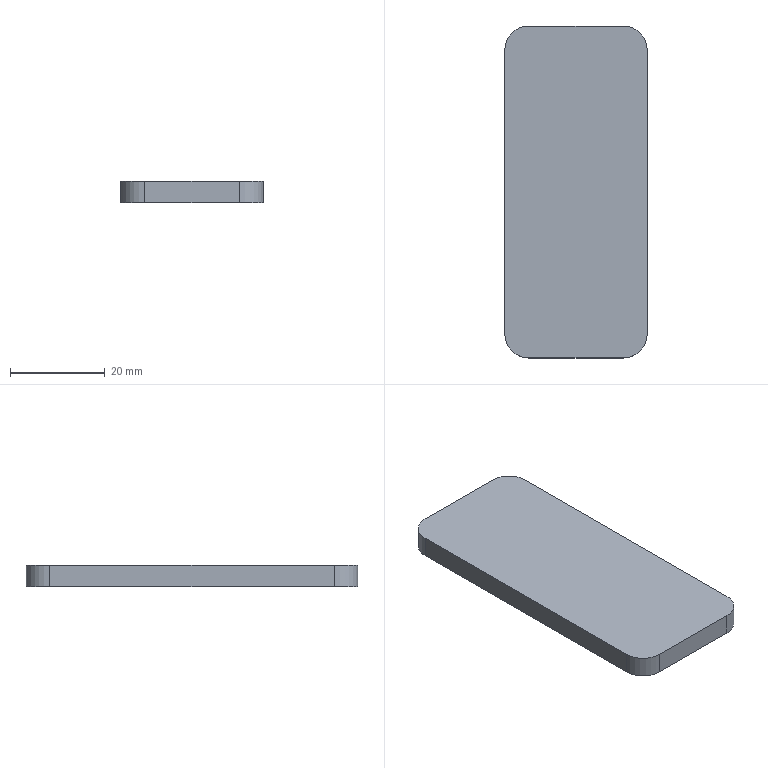Part | SolidWorks | features FlatPattern 1, SMBaseFlange 1, SheetMetal 1 | 1 solid | 10 faces | box 30 x 70 x 4.5 mm | volume 9353 mm3 | plane 6 | cylinder 4 | commonest cylinder face diameters 10 x4
STEP:
#1=CARTESIAN_POINT('',(-15.,-30.,0.));
#2=VERTEX_POINT('',#1);
#3=CARTESIAN_POINT('',(-10.,-35.,0.));
#4=VERTEX_POINT('',#3);
#5=CARTESIAN_POINT('',(-10.,-30.,0.));
#6=DIRECTION('',(0.,0.,1.));
#7=DIRECTION('',(1.,0.,0.));
#8=AXIS2_PLACEMENT_3D('',#5,#6,#7);
#9=CIRCLE('',#8,5.);
#10=EDGE_CURVE('',#2,#4,#9,.T.);
#11=ORIENTED_EDGE('',*,*,#10,.F.);
#12=CARTESIAN_POINT('',(-15.,-30.,-4.5));
#13=VERTEX_POINT('',#12);
#14=CARTESIAN_POINT('',(-15.,-30.,-4.5));
#15=DIRECTION('',(0.,0.,1.));
#16=VECTOR('',#15,1000.);
#17=LINE('',#14,#16);
#18=EDGE_CURVE('',#13,#2,#17,.T.);
#19=ORIENTED_EDGE('',*,*,#18,.F.);
#20=CARTESIAN_POINT('',(-10.,-35.,-4.5));
#21=VERTEX_POINT('',#20);
#22=CARTESIAN_POINT('',(-10.,-30.,-4.5));
#23=DIRECTION('',(0.,0.,1.));
#24=DIRECTION('',(1.,0.,0.));
#25=AXIS2_PLACEMENT_3D('',#22,#23,#24);
#26=CIRCLE('',#25,5.);
#27=EDGE_CURVE('',#13,#21,#26,.T.);
#28=ORIENTED_EDGE('',*,*,#27,.T.);
#29=CARTESIAN_POINT('',(-10.,-35.,-4.5));
#30=DIRECTION('',(0.,0.,1.));
#31=VECTOR('',#30,1000.);
#32=LINE('',#29,#31);
#33=EDGE_CURVE('',#21,#4,#32,.T.);
#34=ORIENTED_EDGE('',*,*,#33,.T.);
#35=EDGE_LOOP('',(#11,#19,#28,#34));
#36=FACE_OUTER_BOUND('',#35,.T.);
#37=CARTESIAN_POINT('',(-10.,-30.,-4.5));
#38=DIRECTION('',(0.,0.,1.));
#39=DIRECTION('',(1.,0.,0.));
#40=AXIS2_PLACEMENT_3D('',#37,#38,#39);
#41=CYLINDRICAL_SURFACE('',#40,5.);
#42=ADVANCED_FACE('',(#36),#41,.T.);
#43=CARTESIAN_POINT('',(-15.,30.,0.));
#44=VERTEX_POINT('',#43);
#45=CARTESIAN_POINT('',(-15.,30.,0.));
#46=DIRECTION('',(0.,-1.,0.));
#47=VECTOR('',#46,1000.);
#48=LINE('',#45,#47);
#49=EDGE_CURVE('',#44,#2,#48,.T.);
#50=ORIENTED_EDGE('',*,*,#49,.F.);
#51=CARTESIAN_POINT('',(-15.,30.,-4.5));
#52=VERTEX_POINT('',#51);
#53=CARTESIAN_POINT('',(-15.,30.,-4.5));
#54=DIRECTION('',(0.,0.,1.));
#55=VECTOR('',#54,1000.);
#56=LINE('',#53,#55);
#57=EDGE_CURVE('',#52,#44,#56,.T.);
#58=ORIENTED_EDGE('',*,*,#57,.F.);
#59=CARTESIAN_POINT('',(-15.,30.,-4.5));
#60=DIRECTION('',(0.,-1.,0.));
#61=VECTOR('',#60,1000.);
#62=LINE('',#59,#61);
#63=EDGE_CURVE('',#52,#13,#62,.T.);
#64=ORIENTED_EDGE('',*,*,#63,.T.);
#65=ORIENTED_EDGE('',*,*,#18,.T.);
#66=EDGE_LOOP('',(#50,#58,#64,#65));
#67=FACE_OUTER_BOUND('',#66,.T.);
#68=CARTESIAN_POINT('',(-15.,30.,-4.5));
#69=DIRECTION('',(-1.,0.,0.));
#70=DIRECTION('',(0.,0.,1.));
#71=AXIS2_PLACEMENT_3D('',#68,#69,#70);
#72=PLANE('',#71);
#73=ADVANCED_FACE('',(#67),#72,.T.);
#74=CARTESIAN_POINT('',(-10.,35.,0.));
#75=VERTEX_POINT('',#74);
#76=CARTESIAN_POINT('',(-10.,30.,0.));
#77=DIRECTION('',(0.,0.,1.));
#78=DIRECTION('',(1.,0.,0.));
#79=AXIS2_PLACEMENT_3D('',#76,#77,#78);
#80=CIRCLE('',#79,5.);
#81=EDGE_CURVE('',#75,#44,#80,.T.);
#82=ORIENTED_EDGE('',*,*,#81,.F.);
#83=CARTESIAN_POINT('',(-10.,35.,-4.5));
#84=VERTEX_POINT('',#83);
#85=CARTESIAN_POINT('',(-10.,35.,-4.5));
#86=DIRECTION('',(0.,0.,1.));
#87=VECTOR('',#86,1000.);
#88=LINE('',#85,#87);
#89=EDGE_CURVE('',#84,#75,#88,.T.);
#90=ORIENTED_EDGE('',*,*,#89,.F.);
#91=CARTESIAN_POINT('',(-10.,30.,-4.5));
#92=DIRECTION('',(0.,0.,1.));
#93=DIRECTION('',(1.,0.,0.));
#94=AXIS2_PLACEMENT_3D('',#91,#92,#93);
#95=CIRCLE('',#94,5.);
#96=EDGE_CURVE('',#84,#52,#95,.T.);
#97=ORIENTED_EDGE('',*,*,#96,.T.);
#98=ORIENTED_EDGE('',*,*,#57,.T.);
#99=EDGE_LOOP('',(#82,#90,#97,#98));
#100=FACE_OUTER_BOUND('',#99,.T.);
#101=CARTESIAN_POINT('',(-10.,30.,-4.5));
#102=DIRECTION('',(0.,0.,1.));
#103=DIRECTION('',(1.,0.,0.));
#104=AXIS2_PLACEMENT_3D('',#101,#102,#103);
#105=CYLINDRICAL_SURFACE('',#104,5.);
#106=ADVANCED_FACE('',(#100),#105,.T.);
#107=CARTESIAN_POINT('',(10.,35.,0.));
#108=VERTEX_POINT('',#107);
#109=CARTESIAN_POINT('',(-10.,35.,0.));
#110=DIRECTION('',(-1.,0.,0.));
#111=VECTOR('',#110,1000.);
#112=LINE('',#109,#111);
#113=EDGE_CURVE('',#108,#75,#112,.T.);
#114=ORIENTED_EDGE('',*,*,#113,.F.);
#115=CARTESIAN_POINT('',(10.,35.,-4.5));
#116=VERTEX_POINT('',#115);
#117=CARTESIAN_POINT('',(10.,35.,-4.5));
#118=DIRECTION('',(0.,0.,1.));
#119=VECTOR('',#118,1000.);
#120=LINE('',#117,#119);
#121=EDGE_CURVE('',#116,#108,#120,.T.);
#122=ORIENTED_EDGE('',*,*,#121,.F.);
#123=CARTESIAN_POINT('',(-10.,35.,-4.5));
#124=DIRECTION('',(-1.,0.,0.));
#125=VECTOR('',#124,1000.);
#126=LINE('',#123,#125);
#127=EDGE_CURVE('',#116,#84,#126,.T.);
#128=ORIENTED_EDGE('',*,*,#127,.T.);
#129=ORIENTED_EDGE('',*,*,#89,.T.);
#130=EDGE_LOOP('',(#114,#122,#128,#129));
#131=FACE_OUTER_BOUND('',#130,.T.);
#132=CARTESIAN_POINT('',(-10.,35.,-4.5));
#133=DIRECTION('',(0.,1.,0.));
#134=DIRECTION('',(0.,0.,1.));
#135=AXIS2_PLACEMENT_3D('',#132,#133,#134);
#136=PLANE('',#135);
#137=ADVANCED_FACE('',(#131),#136,.T.);
#138=CARTESIAN_POINT('',(15.,30.,0.));
#139=VERTEX_POINT('',#138);
#140=CARTESIAN_POINT('',(10.,30.,0.));
#141=DIRECTION('',(0.,0.,1.));
#142=DIRECTION('',(-1.,0.,0.));
#143=AXIS2_PLACEMENT_3D('',#140,#141,#142);
#144=CIRCLE('',#143,5.);
#145=EDGE_CURVE('',#139,#108,#144,.T.);
#146=ORIENTED_EDGE('',*,*,#145,.F.);
#147=CARTESIAN_POINT('',(15.,30.,-4.5));
#148=VERTEX_POINT('',#147);
#149=CARTESIAN_POINT('',(15.,30.,-4.5));
#150=DIRECTION('',(0.,0.,1.));
#151=VECTOR('',#150,1000.);
#152=LINE('',#149,#151);
#153=EDGE_CURVE('',#148,#139,#152,.T.);
#154=ORIENTED_EDGE('',*,*,#153,.F.);
#155=CARTESIAN_POINT('',(10.,30.,-4.5));
#156=DIRECTION('',(0.,0.,1.));
#157=DIRECTION('',(-1.,0.,0.));
#158=AXIS2_PLACEMENT_3D('',#155,#156,#157);
#159=CIRCLE('',#158,5.);
#160=EDGE_CURVE('',#148,#116,#159,.T.);
#161=ORIENTED_EDGE('',*,*,#160,.T.);
#162=ORIENTED_EDGE('',*,*,#121,.T.);
#163=EDGE_LOOP('',(#146,#154,#161,#162));
#164=FACE_OUTER_BOUND('',#163,.T.);
#165=CARTESIAN_POINT('',(10.,30.,-4.5));
#166=DIRECTION('',(0.,0.,1.));
#167=DIRECTION('',(1.,0.,0.));
#168=AXIS2_PLACEMENT_3D('',#165,#166,#167);
#169=CYLINDRICAL_SURFACE('',#168,5.);
#170=ADVANCED_FACE('',(#164),#169,.T.);
#171=CARTESIAN_POINT('',(15.,-30.,0.));
#172=VERTEX_POINT('',#171);
#173=CARTESIAN_POINT('',(15.,30.,0.));
#174=DIRECTION('',(0.,1.,0.));
#175=VECTOR('',#174,1000.);
#176=LINE('',#173,#175);
#177=EDGE_CURVE('',#172,#139,#176,.T.);
#178=ORIENTED_EDGE('',*,*,#177,.F.);
#179=CARTESIAN_POINT('',(15.,-30.,-4.5));
#180=VERTEX_POINT('',#179);
#181=CARTESIAN_POINT('',(15.,-30.,-4.5));
#182=DIRECTION('',(0.,0.,1.));
#183=VECTOR('',#182,1000.);
#184=LINE('',#181,#183);
#185=EDGE_CURVE('',#180,#172,#184,.T.);
#186=ORIENTED_EDGE('',*,*,#185,.F.);
#187=CARTESIAN_POINT('',(15.,30.,-4.5));
#188=DIRECTION('',(0.,1.,0.));
#189=VECTOR('',#188,1000.);
#190=LINE('',#187,#189);
#191=EDGE_CURVE('',#180,#148,#190,.T.);
#192=ORIENTED_EDGE('',*,*,#191,.T.);
#193=ORIENTED_EDGE('',*,*,#153,.T.);
#194=EDGE_LOOP('',(#178,#186,#192,#193));
#195=FACE_OUTER_BOUND('',#194,.T.);
#196=CARTESIAN_POINT('',(15.,30.,-4.5));
#197=DIRECTION('',(1.,0.,0.));
#198=DIRECTION('',(0.,0.,-1.));
#199=AXIS2_PLACEMENT_3D('',#196,#197,#198);
#200=PLANE('',#199);
#201=ADVANCED_FACE('',(#195),#200,.T.);
#202=CARTESIAN_POINT('',(10.,-35.,0.));
#203=VERTEX_POINT('',#202);
#204=CARTESIAN_POINT('',(10.,-30.,0.));
#205=DIRECTION('',(0.,0.,1.));
#206=DIRECTION('',(1.,0.,0.));
#207=AXIS2_PLACEMENT_3D('',#204,#205,#206);
#208=CIRCLE('',#207,5.);
#209=EDGE_CURVE('',#203,#172,#208,.T.);
#210=ORIENTED_EDGE('',*,*,#209,.F.);
#211=CARTESIAN_POINT('',(10.,-35.,-4.5));
#212=VERTEX_POINT('',#211);
#213=CARTESIAN_POINT('',(10.,-35.,-4.5));
#214=DIRECTION('',(0.,0.,1.));
#215=VECTOR('',#214,1000.);
#216=LINE('',#213,#215);
#217=EDGE_CURVE('',#212,#203,#216,.T.);
#218=ORIENTED_EDGE('',*,*,#217,.F.);
#219=CARTESIAN_POINT('',(10.,-30.,-4.5));
#220=DIRECTION('',(0.,0.,1.));
#221=DIRECTION('',(1.,0.,0.));
#222=AXIS2_PLACEMENT_3D('',#219,#220,#221);
#223=CIRCLE('',#222,5.);
#224=EDGE_CURVE('',#212,#180,#223,.T.);
#225=ORIENTED_EDGE('',*,*,#224,.T.);
#226=ORIENTED_EDGE('',*,*,#185,.T.);
#227=EDGE_LOOP('',(#210,#218,#225,#226));
#228=FACE_OUTER_BOUND('',#227,.T.);
#229=CARTESIAN_POINT('',(10.,-30.,-4.5));
#230=DIRECTION('',(0.,0.,1.));
#231=DIRECTION('',(1.,0.,0.));
#232=AXIS2_PLACEMENT_3D('',#229,#230,#231);
#233=CYLINDRICAL_SURFACE('',#232,5.);
#234=ADVANCED_FACE('',(#228),#233,.T.);
#235=CARTESIAN_POINT('',(-10.,-35.,0.));
#236=DIRECTION('',(1.,0.,0.));
#237=VECTOR('',#236,1000.);
#238=LINE('',#235,#237);
#239=EDGE_CURVE('',#4,#203,#238,.T.);
#240=ORIENTED_EDGE('',*,*,#239,.F.);
#241=ORIENTED_EDGE('',*,*,#33,.F.);
#242=CARTESIAN_POINT('',(-10.,-35.,-4.5));
#243=DIRECTION('',(1.,0.,0.));
#244=VECTOR('',#243,1000.);
#245=LINE('',#242,#244);
#246=EDGE_CURVE('',#21,#212,#245,.T.);
#247=ORIENTED_EDGE('',*,*,#246,.T.);
#248=ORIENTED_EDGE('',*,*,#217,.T.);
#249=EDGE_LOOP('',(#240,#241,#247,#248));
#250=FACE_OUTER_BOUND('',#249,.T.);
#251=CARTESIAN_POINT('',(-10.,-35.,-4.5));
#252=DIRECTION('',(0.,-1.,0.));
#253=DIRECTION('',(0.,0.,-1.));
#254=AXIS2_PLACEMENT_3D('',#251,#252,#253);
#255=PLANE('',#254);
#256=ADVANCED_FACE('',(#250),#255,.T.);
#257=ORIENTED_EDGE('',*,*,#27,.F.);
#258=ORIENTED_EDGE('',*,*,#63,.F.);
#259=ORIENTED_EDGE('',*,*,#96,.F.);
#260=ORIENTED_EDGE('',*,*,#127,.F.);
#261=ORIENTED_EDGE('',*,*,#160,.F.);
#262=ORIENTED_EDGE('',*,*,#191,.F.);
#263=ORIENTED_EDGE('',*,*,#224,.F.);
#264=ORIENTED_EDGE('',*,*,#246,.F.);
#265=EDGE_LOOP('',(#257,#258,#259,#260,#261,#262,#263,#264));
#266=FACE_OUTER_BOUND('',#265,.T.);
#267=CARTESIAN_POINT('',(-10.,-30.,-4.5));
#268=DIRECTION('',(0.,0.,1.));
#269=DIRECTION('',(1.,0.,0.));
#270=AXIS2_PLACEMENT_3D('',#267,#268,#269);
#271=PLANE('',#270);
#272=ADVANCED_FACE('',(#266),#271,.F.);
#273=ORIENTED_EDGE('',*,*,#10,.T.);
#274=ORIENTED_EDGE('',*,*,#239,.T.);
#275=ORIENTED_EDGE('',*,*,#209,.T.);
#276=ORIENTED_EDGE('',*,*,#177,.T.);
#277=ORIENTED_EDGE('',*,*,#145,.T.);
#278=ORIENTED_EDGE('',*,*,#113,.T.);
#279=ORIENTED_EDGE('',*,*,#81,.T.);
#280=ORIENTED_EDGE('',*,*,#49,.T.);
#281=EDGE_LOOP('',(#273,#274,#275,#276,#277,#278,#279,#280));
#282=FACE_OUTER_BOUND('',#281,.T.);
#283=CARTESIAN_POINT('',(-10.,-30.,0.));
#284=DIRECTION('',(0.,0.,1.));
#285=DIRECTION('',(1.,0.,0.));
#286=AXIS2_PLACEMENT_3D('',#283,#284,#285);
#287=PLANE('',#286);
#288=ADVANCED_FACE('',(#282),#287,.T.);
#289=CLOSED_SHELL('',(#42,#73,#106,#137,#170,#201,#234,#256,#272,#288));
#290=MANIFOLD_SOLID_BREP('',#289);
#291=CARTESIAN_POINT('',(0.,0.,0.));
#292=DIRECTION('',(0.,0.,1.));
#293=DIRECTION('',(1.,0.,0.));
#294=AXIS2_PLACEMENT_3D('',#291,#292,#293);
#295=(LENGTH_UNIT()NAMED_UNIT(*)SI_UNIT(.MILLI.,.METRE.));
#296=UNCERTAINTY_MEASURE_WITH_UNIT(LENGTH_MEASURE(0.00001),#295,'','');
#297=(NAMED_UNIT(*)PLANE_ANGLE_UNIT()SI_UNIT($,.RADIAN.));
#298=(NAMED_UNIT(*)SI_UNIT($,.STERADIAN.)SOLID_ANGLE_UNIT());
#299=(GEOMETRIC_REPRESENTATION_CONTEXT(3)GLOBAL_UNCERTAINTY_ASSIGNED_CONTEXT((#296))GLOBAL_UNIT_ASSIGNED_CONTEXT((#295,#297,#298))REPRESENTATION_CONTEXT('',''));
#300=ADVANCED_BREP_SHAPE_REPRESENTATION('',(#290,#294),#299);